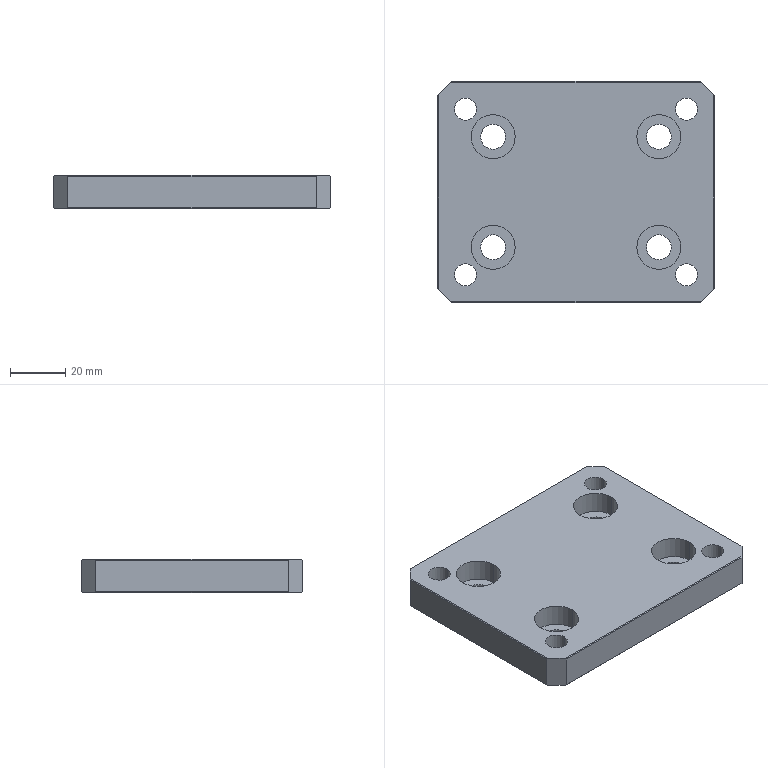Part | NX | 1 solid | 46 faces | box 100 x 80 x 12 mm | volume 85507 mm3 | cylinder 24 | plane 22 | commonest cylinder face diameters 8 x8 9 x8 16 x8
STEP:
#1=CARTESIAN_POINT('',(45.3,0.3,0.));
#2=VERTEX_POINT('',#1);
#3=CARTESIAN_POINT('',(-45.3,0.3,0.));
#4=VERTEX_POINT('',#3);
#5=CARTESIAN_POINT('',(0.,0.3,0.));
#6=DIRECTION('',(-1.,0.,0.));
#7=VECTOR('',#6,1000.);
#8=LINE('',#5,#7);
#9=EDGE_CURVE('',#2,#4,#8,.T.);
#10=ORIENTED_EDGE('',*,*,#9,.T.);
#11=CARTESIAN_POINT('',(-49.7,4.7,0.));
#12=VERTEX_POINT('',#11);
#13=CARTESIAN_POINT('',(-50.,5.,0.));
#14=DIRECTION('',(0.7071,-0.7071,0.));
#15=VECTOR('',#14,1000.);
#16=LINE('',#13,#15);
#17=EDGE_CURVE('',#12,#4,#16,.T.);
#18=ORIENTED_EDGE('',*,*,#17,.F.);
#19=CARTESIAN_POINT('',(-49.7,75.3,0.));
#20=VERTEX_POINT('',#19);
#21=CARTESIAN_POINT('',(-49.7,40.,0.));
#22=DIRECTION('',(0.,1.,0.));
#23=VECTOR('',#22,1000.);
#24=LINE('',#21,#23);
#25=EDGE_CURVE('',#12,#20,#24,.T.);
#26=ORIENTED_EDGE('',*,*,#25,.T.);
#27=CARTESIAN_POINT('',(-45.3,79.7,0.));
#28=VERTEX_POINT('',#27);
#29=CARTESIAN_POINT('',(-45.,80.,0.));
#30=DIRECTION('',(-0.7071,-0.7071,0.));
#31=VECTOR('',#30,1000.);
#32=LINE('',#29,#31);
#33=EDGE_CURVE('',#28,#20,#32,.T.);
#34=ORIENTED_EDGE('',*,*,#33,.F.);
#35=CARTESIAN_POINT('',(45.3,79.7,0.));
#36=VERTEX_POINT('',#35);
#37=CARTESIAN_POINT('',(0.,79.7,0.));
#38=DIRECTION('',(1.,0.,0.));
#39=VECTOR('',#38,1000.);
#40=LINE('',#37,#39);
#41=EDGE_CURVE('',#28,#36,#40,.T.);
#42=ORIENTED_EDGE('',*,*,#41,.T.);
#43=CARTESIAN_POINT('',(49.7,75.3,0.));
#44=VERTEX_POINT('',#43);
#45=CARTESIAN_POINT('',(50.,75.,0.));
#46=DIRECTION('',(-0.7071,0.7071,0.));
#47=VECTOR('',#46,1000.);
#48=LINE('',#45,#47);
#49=EDGE_CURVE('',#44,#36,#48,.T.);
#50=ORIENTED_EDGE('',*,*,#49,.F.);
#51=CARTESIAN_POINT('',(49.7,4.7,0.));
#52=VERTEX_POINT('',#51);
#53=CARTESIAN_POINT('',(49.7,40.,0.));
#54=DIRECTION('',(0.,-1.,0.));
#55=VECTOR('',#54,1000.);
#56=LINE('',#53,#55);
#57=EDGE_CURVE('',#44,#52,#56,.T.);
#58=ORIENTED_EDGE('',*,*,#57,.T.);
#59=CARTESIAN_POINT('',(45.,0.,0.));
#60=DIRECTION('',(0.7071,0.7071,0.));
#61=VECTOR('',#60,1000.);
#62=LINE('',#59,#61);
#63=EDGE_CURVE('',#2,#52,#62,.T.);
#64=ORIENTED_EDGE('',*,*,#63,.F.);
#65=EDGE_LOOP('',(#10,#18,#26,#34,#42,#50,#58,#64));
#66=FACE_BOUND('',#65,.T.);
#67=CARTESIAN_POINT('',(-34.5,60.,0.));
#68=VERTEX_POINT('',#67);
#69=CARTESIAN_POINT('',(-25.5,60.,0.));
#70=VERTEX_POINT('',#69);
#71=CARTESIAN_POINT('',(-30.,60.,0.));
#72=DIRECTION('',(0.,0.,-1.));
#73=DIRECTION('',(-1.,0.,0.));
#74=AXIS2_PLACEMENT_3D('',#71,#72,#73);
#75=CIRCLE('',#74,4.5);
#76=EDGE_CURVE('',#68,#70,#75,.T.);
#77=ORIENTED_EDGE('',*,*,#76,.F.);
#78=CARTESIAN_POINT('',(-30.,60.,0.));
#79=DIRECTION('',(0.,0.,-1.));
#80=DIRECTION('',(-1.,0.,0.));
#81=AXIS2_PLACEMENT_3D('',#78,#79,#80);
#82=CIRCLE('',#81,4.5);
#83=EDGE_CURVE('',#70,#68,#82,.T.);
#84=ORIENTED_EDGE('',*,*,#83,.F.);
#85=EDGE_LOOP('',(#77,#84));
#86=FACE_BOUND('',#85,.T.);
#87=CARTESIAN_POINT('',(25.5,20.,0.));
#88=VERTEX_POINT('',#87);
#89=CARTESIAN_POINT('',(34.5,20.,0.));
#90=VERTEX_POINT('',#89);
#91=CARTESIAN_POINT('',(30.,20.,0.));
#92=DIRECTION('',(0.,0.,-1.));
#93=DIRECTION('',(-1.,0.,0.));
#94=AXIS2_PLACEMENT_3D('',#91,#92,#93);
#95=CIRCLE('',#94,4.5);
#96=EDGE_CURVE('',#88,#90,#95,.T.);
#97=ORIENTED_EDGE('',*,*,#96,.F.);
#98=CARTESIAN_POINT('',(30.,20.,0.));
#99=DIRECTION('',(0.,0.,-1.));
#100=DIRECTION('',(-1.,0.,0.));
#101=AXIS2_PLACEMENT_3D('',#98,#99,#100);
#102=CIRCLE('',#101,4.5);
#103=EDGE_CURVE('',#90,#88,#102,.T.);
#104=ORIENTED_EDGE('',*,*,#103,.F.);
#105=EDGE_LOOP('',(#97,#104));
#106=FACE_BOUND('',#105,.T.);
#107=CARTESIAN_POINT('',(-25.5,20.,0.));
#108=VERTEX_POINT('',#107);
#109=CARTESIAN_POINT('',(-34.5,20.,0.));
#110=VERTEX_POINT('',#109);
#111=CARTESIAN_POINT('',(-30.,20.,0.));
#112=DIRECTION('',(0.,0.,-1.));
#113=DIRECTION('',(-1.,0.,0.));
#114=AXIS2_PLACEMENT_3D('',#111,#112,#113);
#115=CIRCLE('',#114,4.5);
#116=EDGE_CURVE('',#108,#110,#115,.T.);
#117=ORIENTED_EDGE('',*,*,#116,.F.);
#118=CARTESIAN_POINT('',(-30.,20.,0.));
#119=DIRECTION('',(0.,0.,-1.));
#120=DIRECTION('',(-1.,0.,0.));
#121=AXIS2_PLACEMENT_3D('',#118,#119,#120);
#122=CIRCLE('',#121,4.5);
#123=EDGE_CURVE('',#110,#108,#122,.T.);
#124=ORIENTED_EDGE('',*,*,#123,.F.);
#125=EDGE_LOOP('',(#117,#124));
#126=FACE_BOUND('',#125,.T.);
#127=CARTESIAN_POINT('',(36.,10.,0.));
#128=VERTEX_POINT('',#127);
#129=CARTESIAN_POINT('',(44.,10.,0.));
#130=VERTEX_POINT('',#129);
#131=CARTESIAN_POINT('',(40.,10.,0.));
#132=DIRECTION('',(0.,0.,-1.));
#133=DIRECTION('',(1.,0.,0.));
#134=AXIS2_PLACEMENT_3D('',#131,#132,#133);
#135=CIRCLE('',#134,4.);
#136=EDGE_CURVE('',#128,#130,#135,.T.);
#137=ORIENTED_EDGE('',*,*,#136,.F.);
#138=CARTESIAN_POINT('',(40.,10.,0.));
#139=DIRECTION('',(0.,0.,-1.));
#140=DIRECTION('',(1.,0.,0.));
#141=AXIS2_PLACEMENT_3D('',#138,#139,#140);
#142=CIRCLE('',#141,4.);
#143=EDGE_CURVE('',#130,#128,#142,.T.);
#144=ORIENTED_EDGE('',*,*,#143,.F.);
#145=EDGE_LOOP('',(#137,#144));
#146=FACE_BOUND('',#145,.T.);
#147=CARTESIAN_POINT('',(44.,70.,0.));
#148=VERTEX_POINT('',#147);
#149=CARTESIAN_POINT('',(36.,70.,0.));
#150=VERTEX_POINT('',#149);
#151=CARTESIAN_POINT('',(40.,70.,0.));
#152=DIRECTION('',(0.,0.,-1.));
#153=DIRECTION('',(1.,0.,0.));
#154=AXIS2_PLACEMENT_3D('',#151,#152,#153);
#155=CIRCLE('',#154,4.);
#156=EDGE_CURVE('',#148,#150,#155,.T.);
#157=ORIENTED_EDGE('',*,*,#156,.F.);
#158=CARTESIAN_POINT('',(40.,70.,0.));
#159=DIRECTION('',(0.,0.,-1.));
#160=DIRECTION('',(1.,0.,0.));
#161=AXIS2_PLACEMENT_3D('',#158,#159,#160);
#162=CIRCLE('',#161,4.);
#163=EDGE_CURVE('',#150,#148,#162,.T.);
#164=ORIENTED_EDGE('',*,*,#163,.F.);
#165=EDGE_LOOP('',(#157,#164));
#166=FACE_BOUND('',#165,.T.);
#167=CARTESIAN_POINT('',(-36.,10.,0.));
#168=VERTEX_POINT('',#167);
#169=CARTESIAN_POINT('',(-44.,10.,0.));
#170=VERTEX_POINT('',#169);
#171=CARTESIAN_POINT('',(-40.,10.,0.));
#172=DIRECTION('',(0.,0.,-1.));
#173=DIRECTION('',(1.,0.,0.));
#174=AXIS2_PLACEMENT_3D('',#171,#172,#173);
#175=CIRCLE('',#174,4.);
#176=EDGE_CURVE('',#168,#170,#175,.T.);
#177=ORIENTED_EDGE('',*,*,#176,.F.);
#178=CARTESIAN_POINT('',(-40.,10.,0.));
#179=DIRECTION('',(0.,0.,-1.));
#180=DIRECTION('',(1.,0.,0.));
#181=AXIS2_PLACEMENT_3D('',#178,#179,#180);
#182=CIRCLE('',#181,4.);
#183=EDGE_CURVE('',#170,#168,#182,.T.);
#184=ORIENTED_EDGE('',*,*,#183,.F.);
#185=EDGE_LOOP('',(#177,#184));
#186=FACE_BOUND('',#185,.T.);
#187=CARTESIAN_POINT('',(-44.,70.,0.));
#188=VERTEX_POINT('',#187);
#189=CARTESIAN_POINT('',(-36.,70.,0.));
#190=VERTEX_POINT('',#189);
#191=CARTESIAN_POINT('',(-40.,70.,0.));
#192=DIRECTION('',(0.,0.,-1.));
#193=DIRECTION('',(1.,0.,0.));
#194=AXIS2_PLACEMENT_3D('',#191,#192,#193);
#195=CIRCLE('',#194,4.);
#196=EDGE_CURVE('',#188,#190,#195,.T.);
#197=ORIENTED_EDGE('',*,*,#196,.F.);
#198=CARTESIAN_POINT('',(-40.,70.,0.));
#199=DIRECTION('',(0.,0.,-1.));
#200=DIRECTION('',(1.,0.,0.));
#201=AXIS2_PLACEMENT_3D('',#198,#199,#200);
#202=CIRCLE('',#201,4.);
#203=EDGE_CURVE('',#190,#188,#202,.T.);
#204=ORIENTED_EDGE('',*,*,#203,.F.);
#205=EDGE_LOOP('',(#197,#204));
#206=FACE_BOUND('',#205,.T.);
#207=CARTESIAN_POINT('',(34.5,60.,0.));
#208=VERTEX_POINT('',#207);
#209=CARTESIAN_POINT('',(25.5,60.,0.));
#210=VERTEX_POINT('',#209);
#211=CARTESIAN_POINT('',(30.,60.,0.));
#212=DIRECTION('',(0.,0.,-1.));
#213=DIRECTION('',(-1.,0.,0.));
#214=AXIS2_PLACEMENT_3D('',#211,#212,#213);
#215=CIRCLE('',#214,4.5);
#216=EDGE_CURVE('',#208,#210,#215,.T.);
#217=ORIENTED_EDGE('',*,*,#216,.F.);
#218=CARTESIAN_POINT('',(30.,60.,0.));
#219=DIRECTION('',(0.,0.,-1.));
#220=DIRECTION('',(-1.,0.,0.));
#221=AXIS2_PLACEMENT_3D('',#218,#219,#220);
#222=CIRCLE('',#221,4.5);
#223=EDGE_CURVE('',#210,#208,#222,.T.);
#224=ORIENTED_EDGE('',*,*,#223,.F.);
#225=EDGE_LOOP('',(#217,#224));
#226=FACE_BOUND('',#225,.T.);
#227=CARTESIAN_POINT('',(0.,0.,0.));
#228=DIRECTION('',(0.,0.,1.));
#229=DIRECTION('',(1.,0.,0.));
#230=AXIS2_PLACEMENT_3D('',#227,#228,#229);
#231=PLANE('',#230);
#232=ADVANCED_FACE('',(#66,#86,#106,#126,#146,#166,#186,#206,#226),#231,.F.);
#233=CARTESIAN_POINT('',(-50.,5.,0.3));
#234=VERTEX_POINT('',#233);
#235=CARTESIAN_POINT('',(-50.,75.,0.3));
#236=VERTEX_POINT('',#235);
#237=CARTESIAN_POINT('',(-50.,40.,0.3));
#238=DIRECTION('',(0.,1.,0.));
#239=VECTOR('',#238,1000.);
#240=LINE('',#237,#239);
#241=EDGE_CURVE('',#234,#236,#240,.T.);
#242=ORIENTED_EDGE('',*,*,#241,.F.);
#243=CARTESIAN_POINT('',(-50.,5.,11.7));
#244=VERTEX_POINT('',#243);
#245=CARTESIAN_POINT('',(-50.,5.,12.));
#246=DIRECTION('',(0.,0.,-1.));
#247=VECTOR('',#246,1000.);
#248=LINE('',#245,#247);
#249=EDGE_CURVE('',#244,#234,#248,.T.);
#250=ORIENTED_EDGE('',*,*,#249,.F.);
#251=CARTESIAN_POINT('',(-50.,75.,11.7));
#252=VERTEX_POINT('',#251);
#253=CARTESIAN_POINT('',(-50.,40.,11.7));
#254=DIRECTION('',(0.,1.,0.));
#255=VECTOR('',#254,1000.);
#256=LINE('',#253,#255);
#257=EDGE_CURVE('',#244,#252,#256,.T.);
#258=ORIENTED_EDGE('',*,*,#257,.T.);
#259=CARTESIAN_POINT('',(-50.,75.,12.));
#260=DIRECTION('',(0.,0.,-1.));
#261=VECTOR('',#260,1000.);
#262=LINE('',#259,#261);
#263=EDGE_CURVE('',#252,#236,#262,.T.);
#264=ORIENTED_EDGE('',*,*,#263,.T.);
#265=EDGE_LOOP('',(#242,#250,#258,#264));
#266=FACE_BOUND('',#265,.T.);
#267=CARTESIAN_POINT('',(-50.,80.,0.));
#268=DIRECTION('',(-1.,0.,0.));
#269=DIRECTION('',(0.,0.,1.));
#270=AXIS2_PLACEMENT_3D('',#267,#268,#269);
#271=PLANE('',#270);
#272=ADVANCED_FACE('',(#266),#271,.T.);
#273=ORIENTED_EDGE('',*,*,#263,.F.);
#274=CARTESIAN_POINT('',(-49.7,75.3,12.));
#275=VERTEX_POINT('',#274);
#276=CARTESIAN_POINT('',(-61.7,63.3,0.));
#277=DIRECTION('',(0.5774,0.5774,0.5774));
#278=VECTOR('',#277,1000.);
#279=LINE('',#276,#278);
#280=EDGE_CURVE('',#252,#275,#279,.T.);
#281=ORIENTED_EDGE('',*,*,#280,.T.);
#282=CARTESIAN_POINT('',(-45.3,79.7,12.));
#283=VERTEX_POINT('',#282);
#284=CARTESIAN_POINT('',(-50.,75.,12.));
#285=DIRECTION('',(0.7071,0.7071,0.));
#286=VECTOR('',#285,1000.);
#287=LINE('',#284,#286);
#288=EDGE_CURVE('',#275,#283,#287,.T.);
#289=ORIENTED_EDGE('',*,*,#288,.T.);
#290=CARTESIAN_POINT('',(-45.,80.,11.7));
#291=VERTEX_POINT('',#290);
#292=CARTESIAN_POINT('',(-33.3,91.7,0.));
#293=DIRECTION('',(0.5774,0.5774,-0.5774));
#294=VECTOR('',#293,1000.);
#295=LINE('',#292,#294);
#296=EDGE_CURVE('',#283,#291,#295,.T.);
#297=ORIENTED_EDGE('',*,*,#296,.T.);
#298=CARTESIAN_POINT('',(-45.,80.,0.3));
#299=VERTEX_POINT('',#298);
#300=CARTESIAN_POINT('',(-45.,80.,12.));
#301=DIRECTION('',(0.,0.,-1.));
#302=VECTOR('',#301,1000.);
#303=LINE('',#300,#302);
#304=EDGE_CURVE('',#291,#299,#303,.T.);
#305=ORIENTED_EDGE('',*,*,#304,.T.);
#306=CARTESIAN_POINT('',(-45.3,79.7,0.));
#307=DIRECTION('',(0.5774,0.5774,0.5774));
#308=VECTOR('',#307,1000.);
#309=LINE('',#306,#308);
#310=EDGE_CURVE('',#28,#299,#309,.T.);
#311=ORIENTED_EDGE('',*,*,#310,.F.);
#312=ORIENTED_EDGE('',*,*,#33,.T.);
#313=CARTESIAN_POINT('',(-49.7,75.3,0.));
#314=DIRECTION('',(0.5774,0.5774,-0.5774));
#315=VECTOR('',#314,1000.);
#316=LINE('',#313,#315);
#317=EDGE_CURVE('',#236,#20,#316,.T.);
#318=ORIENTED_EDGE('',*,*,#317,.F.);
#319=EDGE_LOOP('',(#273,#281,#289,#297,#305,#311,#312,#318));
#320=FACE_BOUND('',#319,.T.);
#321=CARTESIAN_POINT('',(-50.,75.,0.));
#322=DIRECTION('',(-0.7071,0.7071,0.));
#323=DIRECTION('',(0.,0.,1.));
#324=AXIS2_PLACEMENT_3D('',#321,#322,#323);
#325=PLANE('',#324);
#326=ADVANCED_FACE('',(#320),#325,.T.);
#327=CARTESIAN_POINT('',(45.,80.,0.3));
#328=VERTEX_POINT('',#327);
#329=CARTESIAN_POINT('',(0.,80.,0.3));
#330=DIRECTION('',(1.,0.,0.));
#331=VECTOR('',#330,1000.);
#332=LINE('',#329,#331);
#333=EDGE_CURVE('',#299,#328,#332,.T.);
#334=ORIENTED_EDGE('',*,*,#333,.F.);
#335=ORIENTED_EDGE('',*,*,#304,.F.);
#336=CARTESIAN_POINT('',(45.,80.,11.7));
#337=VERTEX_POINT('',#336);
#338=CARTESIAN_POINT('',(0.,80.,11.7));
#339=DIRECTION('',(1.,0.,0.));
#340=VECTOR('',#339,1000.);
#341=LINE('',#338,#340);
#342=EDGE_CURVE('',#291,#337,#341,.T.);
#343=ORIENTED_EDGE('',*,*,#342,.T.);
#344=CARTESIAN_POINT('',(45.,80.,12.));
#345=DIRECTION('',(0.,0.,-1.));
#346=VECTOR('',#345,1000.);
#347=LINE('',#344,#346);
#348=EDGE_CURVE('',#337,#328,#347,.T.);
#349=ORIENTED_EDGE('',*,*,#348,.T.);
#350=EDGE_LOOP('',(#334,#335,#343,#349));
#351=FACE_BOUND('',#350,.T.);
#352=CARTESIAN_POINT('',(50.,80.,0.));
#353=DIRECTION('',(0.,1.,0.));
#354=DIRECTION('',(1.,0.,0.));
#355=AXIS2_PLACEMENT_3D('',#352,#353,#354);
#356=PLANE('',#355);
#357=ADVANCED_FACE('',(#351),#356,.T.);
#358=ORIENTED_EDGE('',*,*,#348,.F.);
#359=CARTESIAN_POINT('',(45.3,79.7,12.));
#360=VERTEX_POINT('',#359);
#361=CARTESIAN_POINT('',(33.3,91.7,0.));
#362=DIRECTION('',(0.5774,-0.5774,0.5774));
#363=VECTOR('',#362,1000.);
#364=LINE('',#361,#363);
#365=EDGE_CURVE('',#337,#360,#364,.T.);
#366=ORIENTED_EDGE('',*,*,#365,.T.);
#367=CARTESIAN_POINT('',(49.7,75.3,12.));
#368=VERTEX_POINT('',#367);
#369=CARTESIAN_POINT('',(45.,80.,12.));
#370=DIRECTION('',(0.7071,-0.7071,0.));
#371=VECTOR('',#370,1000.);
#372=LINE('',#369,#371);
#373=EDGE_CURVE('',#360,#368,#372,.T.);
#374=ORIENTED_EDGE('',*,*,#373,.T.);
#375=CARTESIAN_POINT('',(50.,75.,11.7));
#376=VERTEX_POINT('',#375);
#377=CARTESIAN_POINT('',(61.7,63.3,0.));
#378=DIRECTION('',(0.5774,-0.5774,-0.5774));
#379=VECTOR('',#378,1000.);
#380=LINE('',#377,#379);
#381=EDGE_CURVE('',#368,#376,#380,.T.);
#382=ORIENTED_EDGE('',*,*,#381,.T.);
#383=CARTESIAN_POINT('',(50.,75.,0.3));
#384=VERTEX_POINT('',#383);
#385=CARTESIAN_POINT('',(50.,75.,12.));
#386=DIRECTION('',(0.,0.,-1.));
#387=VECTOR('',#386,1000.);
#388=LINE('',#385,#387);
#389=EDGE_CURVE('',#376,#384,#388,.T.);
#390=ORIENTED_EDGE('',*,*,#389,.T.);
#391=CARTESIAN_POINT('',(49.7,75.3,0.));
#392=DIRECTION('',(0.5774,-0.5774,0.5774));
#393=VECTOR('',#392,1000.);
#394=LINE('',#391,#393);
#395=EDGE_CURVE('',#44,#384,#394,.T.);
#396=ORIENTED_EDGE('',*,*,#395,.F.);
#397=ORIENTED_EDGE('',*,*,#49,.T.);
#398=CARTESIAN_POINT('',(45.3,79.7,0.));
#399=DIRECTION('',(0.5774,-0.5774,-0.5774));
#400=VECTOR('',#399,1000.);
#401=LINE('',#398,#400);
#402=EDGE_CURVE('',#328,#36,#401,.T.);
#403=ORIENTED_EDGE('',*,*,#402,.F.);
#404=EDGE_LOOP('',(#358,#366,#374,#382,#390,#396,#397,#403));
#405=FACE_BOUND('',#404,.T.);
#406=CARTESIAN_POINT('',(45.,80.,0.));
#407=DIRECTION('',(0.7071,0.7071,0.));
#408=DIRECTION('',(0.,0.,-1.));
#409=AXIS2_PLACEMENT_3D('',#406,#407,#408);
#410=PLANE('',#409);
#411=ADVANCED_FACE('',(#405),#410,.T.);
#412=CARTESIAN_POINT('',(50.,5.,0.3));
#413=VERTEX_POINT('',#412);
#414=CARTESIAN_POINT('',(50.,40.,0.3));
#415=DIRECTION('',(0.,-1.,0.));
#416=VECTOR('',#415,1000.);
#417=LINE('',#414,#416);
#418=EDGE_CURVE('',#384,#413,#417,.T.);
#419=ORIENTED_EDGE('',*,*,#418,.F.);
#420=ORIENTED_EDGE('',*,*,#389,.F.);
#421=CARTESIAN_POINT('',(50.,5.,11.7));
#422=VERTEX_POINT('',#421);
#423=CARTESIAN_POINT('',(50.,40.,11.7));
#424=DIRECTION('',(0.,-1.,0.));
#425=VECTOR('',#424,1000.);
#426=LINE('',#423,#425);
#427=EDGE_CURVE('',#376,#422,#426,.T.);
#428=ORIENTED_EDGE('',*,*,#427,.T.);
#429=CARTESIAN_POINT('',(50.,5.,12.));
#430=DIRECTION('',(0.,0.,-1.));
#431=VECTOR('',#430,1000.);
#432=LINE('',#429,#431);
#433=EDGE_CURVE('',#422,#413,#432,.T.);
#434=ORIENTED_EDGE('',*,*,#433,.T.);
#435=EDGE_LOOP('',(#419,#420,#428,#434));
#436=FACE_BOUND('',#435,.T.);
#437=CARTESIAN_POINT('',(50.,0.,0.));
#438=DIRECTION('',(1.,0.,0.));
#439=DIRECTION('',(0.,1.,0.));
#440=AXIS2_PLACEMENT_3D('',#437,#438,#439);
#441=PLANE('',#440);
#442=ADVANCED_FACE('',(#436),#441,.T.);
#443=ORIENTED_EDGE('',*,*,#433,.F.);
#444=CARTESIAN_POINT('',(49.7,4.7,12.));
#445=VERTEX_POINT('',#444);
#446=CARTESIAN_POINT('',(61.7,16.7,0.));
#447=DIRECTION('',(-0.5774,-0.5774,0.5774));
#448=VECTOR('',#447,1000.);
#449=LINE('',#446,#448);
#450=EDGE_CURVE('',#422,#445,#449,.T.);
#451=ORIENTED_EDGE('',*,*,#450,.T.);
#452=CARTESIAN_POINT('',(45.3,0.3,12.));
#453=VERTEX_POINT('',#452);
#454=CARTESIAN_POINT('',(50.,5.,12.));
#455=DIRECTION('',(-0.7071,-0.7071,0.));
#456=VECTOR('',#455,1000.);
#457=LINE('',#454,#456);
#458=EDGE_CURVE('',#445,#453,#457,.T.);
#459=ORIENTED_EDGE('',*,*,#458,.T.);
#460=CARTESIAN_POINT('',(45.,0.,11.7));
#461=VERTEX_POINT('',#460);
#462=CARTESIAN_POINT('',(33.3,-11.7,0.));
#463=DIRECTION('',(-0.5774,-0.5774,-0.5774));
#464=VECTOR('',#463,1000.);
#465=LINE('',#462,#464);
#466=EDGE_CURVE('',#453,#461,#465,.T.);
#467=ORIENTED_EDGE('',*,*,#466,.T.);
#468=CARTESIAN_POINT('',(45.,0.,0.3));
#469=VERTEX_POINT('',#468);
#470=CARTESIAN_POINT('',(45.,0.,12.));
#471=DIRECTION('',(0.,0.,-1.));
#472=VECTOR('',#471,1000.);
#473=LINE('',#470,#472);
#474=EDGE_CURVE('',#461,#469,#473,.T.);
#475=ORIENTED_EDGE('',*,*,#474,.T.);
#476=CARTESIAN_POINT('',(45.3,0.3,0.));
#477=DIRECTION('',(-0.5774,-0.5774,0.5774));
#478=VECTOR('',#477,1000.);
#479=LINE('',#476,#478);
#480=EDGE_CURVE('',#2,#469,#479,.T.);
#481=ORIENTED_EDGE('',*,*,#480,.F.);
#482=ORIENTED_EDGE('',*,*,#63,.T.);
#483=CARTESIAN_POINT('',(49.7,4.7,0.));
#484=DIRECTION('',(-0.5774,-0.5774,-0.5774));
#485=VECTOR('',#484,1000.);
#486=LINE('',#483,#485);
#487=EDGE_CURVE('',#413,#52,#486,.T.);
#488=ORIENTED_EDGE('',*,*,#487,.F.);
#489=EDGE_LOOP('',(#443,#451,#459,#467,#475,#481,#482,#488));
#490=FACE_BOUND('',#489,.T.);
#491=CARTESIAN_POINT('',(50.,5.,0.));
#492=DIRECTION('',(0.7071,-0.7071,0.));
#493=DIRECTION('',(0.,0.,-1.));
#494=AXIS2_PLACEMENT_3D('',#491,#492,#493);
#495=PLANE('',#494);
#496=ADVANCED_FACE('',(#490),#495,.T.);
#497=CARTESIAN_POINT('',(-45.,0.,0.3));
#498=VERTEX_POINT('',#497);
#499=CARTESIAN_POINT('',(0.,0.,0.3));
#500=DIRECTION('',(-1.,0.,0.));
#501=VECTOR('',#500,1000.);
#502=LINE('',#499,#501);
#503=EDGE_CURVE('',#469,#498,#502,.T.);
#504=ORIENTED_EDGE('',*,*,#503,.F.);
#505=ORIENTED_EDGE('',*,*,#474,.F.);
#506=CARTESIAN_POINT('',(-45.,0.,11.7));
#507=VERTEX_POINT('',#506);
#508=CARTESIAN_POINT('',(0.,0.,11.7));
#509=DIRECTION('',(-1.,0.,0.));
#510=VECTOR('',#509,1000.);
#511=LINE('',#508,#510);
#512=EDGE_CURVE('',#461,#507,#511,.T.);
#513=ORIENTED_EDGE('',*,*,#512,.T.);
#514=CARTESIAN_POINT('',(-45.,0.,12.));
#515=DIRECTION('',(0.,0.,-1.));
#516=VECTOR('',#515,1000.);
#517=LINE('',#514,#516);
#518=EDGE_CURVE('',#507,#498,#517,.T.);
#519=ORIENTED_EDGE('',*,*,#518,.T.);
#520=EDGE_LOOP('',(#504,#505,#513,#519));
#521=FACE_BOUND('',#520,.T.);
#522=CARTESIAN_POINT('',(-50.,0.,0.));
#523=DIRECTION('',(0.,-1.,0.));
#524=DIRECTION('',(0.,0.,-1.));
#525=AXIS2_PLACEMENT_3D('',#522,#523,#524);
#526=PLANE('',#525);
#527=ADVANCED_FACE('',(#521),#526,.T.);
#528=ORIENTED_EDGE('',*,*,#518,.F.);
#529=CARTESIAN_POINT('',(-45.3,0.3,12.));
#530=VERTEX_POINT('',#529);
#531=CARTESIAN_POINT('',(-33.3,-11.7,0.));
#532=DIRECTION('',(-0.5774,0.5774,0.5774));
#533=VECTOR('',#532,1000.);
#534=LINE('',#531,#533);
#535=EDGE_CURVE('',#507,#530,#534,.T.);
#536=ORIENTED_EDGE('',*,*,#535,.T.);
#537=CARTESIAN_POINT('',(-49.7,4.7,12.));
#538=VERTEX_POINT('',#537);
#539=CARTESIAN_POINT('',(-45.,0.,12.));
#540=DIRECTION('',(-0.7071,0.7071,0.));
#541=VECTOR('',#540,1000.);
#542=LINE('',#539,#541);
#543=EDGE_CURVE('',#530,#538,#542,.T.);
#544=ORIENTED_EDGE('',*,*,#543,.T.);
#545=CARTESIAN_POINT('',(-61.7,16.7,0.));
#546=DIRECTION('',(-0.5774,0.5774,-0.5774));
#547=VECTOR('',#546,1000.);
#548=LINE('',#545,#547);
#549=EDGE_CURVE('',#538,#244,#548,.T.);
#550=ORIENTED_EDGE('',*,*,#549,.T.);
#551=ORIENTED_EDGE('',*,*,#249,.T.);
#552=CARTESIAN_POINT('',(-49.7,4.7,0.));
#553=DIRECTION('',(-0.5774,0.5774,0.5774));
#554=VECTOR('',#553,1000.);
#555=LINE('',#552,#554);
#556=EDGE_CURVE('',#12,#234,#555,.T.);
#557=ORIENTED_EDGE('',*,*,#556,.F.);
#558=ORIENTED_EDGE('',*,*,#17,.T.);
#559=CARTESIAN_POINT('',(-45.3,0.3,0.));
#560=DIRECTION('',(-0.5774,0.5774,-0.5774));
#561=VECTOR('',#560,1000.);
#562=LINE('',#559,#561);
#563=EDGE_CURVE('',#498,#4,#562,.T.);
#564=ORIENTED_EDGE('',*,*,#563,.F.);
#565=EDGE_LOOP('',(#528,#536,#544,#550,#551,#557,#558,#564));
#566=FACE_BOUND('',#565,.T.);
#567=CARTESIAN_POINT('',(-45.,0.,0.));
#568=DIRECTION('',(-0.7071,-0.7071,0.));
#569=DIRECTION('',(-0.7071,0.7071,0.));
#570=AXIS2_PLACEMENT_3D('',#567,#568,#569);
#571=PLANE('',#570);
#572=ADVANCED_FACE('',(#566),#571,.T.);
#573=CARTESIAN_POINT('',(0.,0.3,12.));
#574=DIRECTION('',(-1.,0.,0.));
#575=VECTOR('',#574,1000.);
#576=LINE('',#573,#575);
#577=EDGE_CURVE('',#453,#530,#576,.T.);
#578=ORIENTED_EDGE('',*,*,#577,.F.);
#579=ORIENTED_EDGE('',*,*,#458,.F.);
#580=CARTESIAN_POINT('',(49.7,40.,12.));
#581=DIRECTION('',(0.,-1.,0.));
#582=VECTOR('',#581,1000.);
#583=LINE('',#580,#582);
#584=EDGE_CURVE('',#368,#445,#583,.T.);
#585=ORIENTED_EDGE('',*,*,#584,.F.);
#586=ORIENTED_EDGE('',*,*,#373,.F.);
#587=CARTESIAN_POINT('',(0.,79.7,12.));
#588=DIRECTION('',(1.,0.,0.));
#589=VECTOR('',#588,1000.);
#590=LINE('',#587,#589);
#591=EDGE_CURVE('',#283,#360,#590,.T.);
#592=ORIENTED_EDGE('',*,*,#591,.F.);
#593=ORIENTED_EDGE('',*,*,#288,.F.);
#594=CARTESIAN_POINT('',(-49.7,40.,12.));
#595=DIRECTION('',(0.,1.,0.));
#596=VECTOR('',#595,1000.);
#597=LINE('',#594,#596);
#598=EDGE_CURVE('',#538,#275,#597,.T.);
#599=ORIENTED_EDGE('',*,*,#598,.F.);
#600=ORIENTED_EDGE('',*,*,#543,.F.);
#601=EDGE_LOOP('',(#578,#579,#585,#586,#592,#593,#599,#600));
#602=FACE_BOUND('',#601,.T.);
#603=CARTESIAN_POINT('',(-38.,60.,12.));
#604=VERTEX_POINT('',#603);
#605=CARTESIAN_POINT('',(-22.,60.,12.));
#606=VERTEX_POINT('',#605);
#607=CARTESIAN_POINT('',(-30.,60.,12.));
#608=DIRECTION('',(0.,0.,1.));
#609=DIRECTION('',(1.,0.,0.));
#610=AXIS2_PLACEMENT_3D('',#607,#608,#609);
#611=CIRCLE('',#610,8.);
#612=EDGE_CURVE('',#604,#606,#611,.T.);
#613=ORIENTED_EDGE('',*,*,#612,.F.);
#614=CARTESIAN_POINT('',(-30.,60.,12.));
#615=DIRECTION('',(0.,0.,1.));
#616=DIRECTION('',(1.,0.,0.));
#617=AXIS2_PLACEMENT_3D('',#614,#615,#616);
#618=CIRCLE('',#617,8.);
#619=EDGE_CURVE('',#606,#604,#618,.T.);
#620=ORIENTED_EDGE('',*,*,#619,.F.);
#621=EDGE_LOOP('',(#613,#620));
#622=FACE_BOUND('',#621,.T.);
#623=CARTESIAN_POINT('',(38.,20.,12.));
#624=VERTEX_POINT('',#623);
#625=CARTESIAN_POINT('',(22.,20.,12.));
#626=VERTEX_POINT('',#625);
#627=CARTESIAN_POINT('',(30.,20.,12.));
#628=DIRECTION('',(0.,0.,1.));
#629=DIRECTION('',(1.,0.,0.));
#630=AXIS2_PLACEMENT_3D('',#627,#628,#629);
#631=CIRCLE('',#630,8.);
#632=EDGE_CURVE('',#624,#626,#631,.T.);
#633=ORIENTED_EDGE('',*,*,#632,.F.);
#634=CARTESIAN_POINT('',(30.,20.,12.));
#635=DIRECTION('',(0.,0.,1.));
#636=DIRECTION('',(1.,0.,0.));
#637=AXIS2_PLACEMENT_3D('',#634,#635,#636);
#638=CIRCLE('',#637,8.);
#639=EDGE_CURVE('',#626,#624,#638,.T.);
#640=ORIENTED_EDGE('',*,*,#639,.F.);
#641=EDGE_LOOP('',(#633,#640));
#642=FACE_BOUND('',#641,.T.);
#643=CARTESIAN_POINT('',(-38.,20.,12.));
#644=VERTEX_POINT('',#643);
#645=CARTESIAN_POINT('',(-22.,20.,12.));
#646=VERTEX_POINT('',#645);
#647=CARTESIAN_POINT('',(-30.,20.,12.));
#648=DIRECTION('',(0.,0.,1.));
#649=DIRECTION('',(1.,0.,0.));
#650=AXIS2_PLACEMENT_3D('',#647,#648,#649);
#651=CIRCLE('',#650,8.);
#652=EDGE_CURVE('',#644,#646,#651,.T.);
#653=ORIENTED_EDGE('',*,*,#652,.F.);
#654=CARTESIAN_POINT('',(-30.,20.,12.));
#655=DIRECTION('',(0.,0.,1.));
#656=DIRECTION('',(1.,0.,0.));
#657=AXIS2_PLACEMENT_3D('',#654,#655,#656);
#658=CIRCLE('',#657,8.);
#659=EDGE_CURVE('',#646,#644,#658,.T.);
#660=ORIENTED_EDGE('',*,*,#659,.F.);
#661=EDGE_LOOP('',(#653,#660));
#662=FACE_BOUND('',#661,.T.);
#663=CARTESIAN_POINT('',(44.,10.,12.));
#664=VERTEX_POINT('',#663);
#665=CARTESIAN_POINT('',(36.,10.,12.));
#666=VERTEX_POINT('',#665);
#667=CARTESIAN_POINT('',(40.,10.,12.));
#668=DIRECTION('',(0.,0.,1.));
#669=DIRECTION('',(-1.,0.,0.));
#670=AXIS2_PLACEMENT_3D('',#667,#668,#669);
#671=CIRCLE('',#670,4.);
#672=EDGE_CURVE('',#664,#666,#671,.T.);
#673=ORIENTED_EDGE('',*,*,#672,.F.);
#674=CARTESIAN_POINT('',(40.,10.,12.));
#675=DIRECTION('',(0.,0.,1.));
#676=DIRECTION('',(-1.,0.,0.));
#677=AXIS2_PLACEMENT_3D('',#674,#675,#676);
#678=CIRCLE('',#677,4.);
#679=EDGE_CURVE('',#666,#664,#678,.T.);
#680=ORIENTED_EDGE('',*,*,#679,.F.);
#681=EDGE_LOOP('',(#673,#680));
#682=FACE_BOUND('',#681,.T.);
#683=CARTESIAN_POINT('',(44.,70.,12.));
#684=VERTEX_POINT('',#683);
#685=CARTESIAN_POINT('',(36.,70.,12.));
#686=VERTEX_POINT('',#685);
#687=CARTESIAN_POINT('',(40.,70.,12.));
#688=DIRECTION('',(0.,0.,1.));
#689=DIRECTION('',(-1.,0.,0.));
#690=AXIS2_PLACEMENT_3D('',#687,#688,#689);
#691=CIRCLE('',#690,4.);
#692=EDGE_CURVE('',#684,#686,#691,.T.);
#693=ORIENTED_EDGE('',*,*,#692,.F.);
#694=CARTESIAN_POINT('',(40.,70.,12.));
#695=DIRECTION('',(0.,0.,1.));
#696=DIRECTION('',(-1.,0.,0.));
#697=AXIS2_PLACEMENT_3D('',#694,#695,#696);
#698=CIRCLE('',#697,4.);
#699=EDGE_CURVE('',#686,#684,#698,.T.);
#700=ORIENTED_EDGE('',*,*,#699,.F.);
#701=EDGE_LOOP('',(#693,#700));
#702=FACE_BOUND('',#701,.T.);
#703=CARTESIAN_POINT('',(-44.,10.,12.));
#704=VERTEX_POINT('',#703);
#705=CARTESIAN_POINT('',(-36.,10.,12.));
#706=VERTEX_POINT('',#705);
#707=CARTESIAN_POINT('',(-40.,10.,12.));
#708=DIRECTION('',(0.,0.,1.));
#709=DIRECTION('',(-1.,0.,0.));
#710=AXIS2_PLACEMENT_3D('',#707,#708,#709);
#711=CIRCLE('',#710,4.);
#712=EDGE_CURVE('',#704,#706,#711,.T.);
#713=ORIENTED_EDGE('',*,*,#712,.F.);
#714=CARTESIAN_POINT('',(-40.,10.,12.));
#715=DIRECTION('',(0.,0.,1.));
#716=DIRECTION('',(-1.,0.,0.));
#717=AXIS2_PLACEMENT_3D('',#714,#715,#716);
#718=CIRCLE('',#717,4.);
#719=EDGE_CURVE('',#706,#704,#718,.T.);
#720=ORIENTED_EDGE('',*,*,#719,.F.);
#721=EDGE_LOOP('',(#713,#720));
#722=FACE_BOUND('',#721,.T.);
#723=CARTESIAN_POINT('',(-44.,70.,12.));
#724=VERTEX_POINT('',#723);
#725=CARTESIAN_POINT('',(-36.,70.,12.));
#726=VERTEX_POINT('',#725);
#727=CARTESIAN_POINT('',(-40.,70.,12.));
#728=DIRECTION('',(0.,0.,1.));
#729=DIRECTION('',(-1.,0.,0.));
#730=AXIS2_PLACEMENT_3D('',#727,#728,#729);
#731=CIRCLE('',#730,4.);
#732=EDGE_CURVE('',#724,#726,#731,.T.);
#733=ORIENTED_EDGE('',*,*,#732,.F.);
#734=CARTESIAN_POINT('',(-40.,70.,12.));
#735=DIRECTION('',(0.,0.,1.));
#736=DIRECTION('',(-1.,0.,0.));
#737=AXIS2_PLACEMENT_3D('',#734,#735,#736);
#738=CIRCLE('',#737,4.);
#739=EDGE_CURVE('',#726,#724,#738,.T.);
#740=ORIENTED_EDGE('',*,*,#739,.F.);
#741=EDGE_LOOP('',(#733,#740));
#742=FACE_BOUND('',#741,.T.);
#743=CARTESIAN_POINT('',(38.,60.,12.));
#744=VERTEX_POINT('',#743);
#745=CARTESIAN_POINT('',(22.,60.,12.));
#746=VERTEX_POINT('',#745);
#747=CARTESIAN_POINT('',(30.,60.,12.));
#748=DIRECTION('',(0.,0.,1.));
#749=DIRECTION('',(1.,0.,0.));
#750=AXIS2_PLACEMENT_3D('',#747,#748,#749);
#751=CIRCLE('',#750,8.);
#752=EDGE_CURVE('',#744,#746,#751,.T.);
#753=ORIENTED_EDGE('',*,*,#752,.F.);
#754=CARTESIAN_POINT('',(30.,60.,12.));
#755=DIRECTION('',(0.,0.,1.));
#756=DIRECTION('',(1.,0.,0.));
#757=AXIS2_PLACEMENT_3D('',#754,#755,#756);
#758=CIRCLE('',#757,8.);
#759=EDGE_CURVE('',#746,#744,#758,.T.);
#760=ORIENTED_EDGE('',*,*,#759,.F.);
#761=EDGE_LOOP('',(#753,#760));
#762=FACE_BOUND('',#761,.T.);
#763=CARTESIAN_POINT('',(0.,0.,12.));
#764=DIRECTION('',(0.,0.,1.));
#765=DIRECTION('',(1.,0.,0.));
#766=AXIS2_PLACEMENT_3D('',#763,#764,#765);
#767=PLANE('',#766);
#768=ADVANCED_FACE('',(#602,#622,#642,#662,#682,#702,#722,#742,#762),#767,.T.);
#769=CARTESIAN_POINT('',(22.,60.,4.));
#770=VERTEX_POINT('',#769);
#771=CARTESIAN_POINT('',(38.,60.,4.));
#772=VERTEX_POINT('',#771);
#773=CARTESIAN_POINT('',(30.,60.,4.));
#774=DIRECTION('',(0.,0.,-1.));
#775=DIRECTION('',(1.,0.,0.));
#776=AXIS2_PLACEMENT_3D('',#773,#774,#775);
#777=CIRCLE('',#776,8.);
#778=EDGE_CURVE('',#770,#772,#777,.T.);
#779=ORIENTED_EDGE('',*,*,#778,.T.);
#780=CARTESIAN_POINT('',(38.,60.,-1.86));
#781=DIRECTION('',(0.,0.,1.));
#782=VECTOR('',#781,1000.);
#783=LINE('',#780,#782);
#784=EDGE_CURVE('',#744,#772,#783,.F.);
#785=ORIENTED_EDGE('',*,*,#784,.F.);
#786=ORIENTED_EDGE('',*,*,#752,.T.);
#787=CARTESIAN_POINT('',(22.,60.,-1.86));
#788=DIRECTION('',(0.,0.,1.));
#789=VECTOR('',#788,1000.);
#790=LINE('',#787,#789);
#791=EDGE_CURVE('',#746,#770,#790,.F.);
#792=ORIENTED_EDGE('',*,*,#791,.T.);
#793=EDGE_LOOP('',(#779,#785,#786,#792));
#794=FACE_BOUND('',#793,.T.);
#795=CARTESIAN_POINT('',(30.,60.,-1.86));
#796=DIRECTION('',(0.,0.,1.));
#797=DIRECTION('',(-1.,0.,0.));
#798=AXIS2_PLACEMENT_3D('',#795,#796,#797);
#799=CYLINDRICAL_SURFACE('',#798,8.);
#800=ADVANCED_FACE('',(#794),#799,.F.);
#801=ORIENTED_EDGE('',*,*,#136,.T.);
#802=CARTESIAN_POINT('',(44.,10.,12.));
#803=DIRECTION('',(0.,0.,-1.));
#804=VECTOR('',#803,1000.);
#805=LINE('',#802,#804);
#806=EDGE_CURVE('',#130,#664,#805,.F.);
#807=ORIENTED_EDGE('',*,*,#806,.T.);
#808=ORIENTED_EDGE('',*,*,#672,.T.);
#809=CARTESIAN_POINT('',(36.,10.,12.));
#810=DIRECTION('',(0.,0.,-1.));
#811=VECTOR('',#810,1000.);
#812=LINE('',#809,#811);
#813=EDGE_CURVE('',#128,#666,#812,.F.);
#814=ORIENTED_EDGE('',*,*,#813,.F.);
#815=EDGE_LOOP('',(#801,#807,#808,#814));
#816=FACE_BOUND('',#815,.T.);
#817=CARTESIAN_POINT('',(40.,10.,12.));
#818=DIRECTION('',(0.,0.,-1.));
#819=DIRECTION('',(-1.,0.,0.));
#820=AXIS2_PLACEMENT_3D('',#817,#818,#819);
#821=CYLINDRICAL_SURFACE('',#820,4.);
#822=ADVANCED_FACE('',(#816),#821,.F.);
#823=ORIENTED_EDGE('',*,*,#778,.F.);
#824=CARTESIAN_POINT('',(30.,60.,4.));
#825=DIRECTION('',(0.,0.,-1.));
#826=DIRECTION('',(1.,0.,0.));
#827=AXIS2_PLACEMENT_3D('',#824,#825,#826);
#828=CIRCLE('',#827,8.);
#829=EDGE_CURVE('',#772,#770,#828,.T.);
#830=ORIENTED_EDGE('',*,*,#829,.F.);
#831=EDGE_LOOP('',(#823,#830));
#832=FACE_BOUND('',#831,.T.);
#833=CARTESIAN_POINT('',(25.5,60.,4.));
#834=VERTEX_POINT('',#833);
#835=CARTESIAN_POINT('',(34.5,60.,4.));
#836=VERTEX_POINT('',#835);
#837=CARTESIAN_POINT('',(30.,60.,4.));
#838=DIRECTION('',(0.,0.,1.));
#839=DIRECTION('',(-1.,0.,0.));
#840=AXIS2_PLACEMENT_3D('',#837,#838,#839);
#841=CIRCLE('',#840,4.5);
#842=EDGE_CURVE('',#834,#836,#841,.T.);
#843=ORIENTED_EDGE('',*,*,#842,.F.);
#844=CARTESIAN_POINT('',(30.,60.,4.));
#845=DIRECTION('',(0.,0.,1.));
#846=DIRECTION('',(-1.,0.,0.));
#847=AXIS2_PLACEMENT_3D('',#844,#845,#846);
#848=CIRCLE('',#847,4.5);
#849=EDGE_CURVE('',#836,#834,#848,.T.);
#850=ORIENTED_EDGE('',*,*,#849,.F.);
#851=EDGE_LOOP('',(#843,#850));
#852=FACE_BOUND('',#851,.T.);
#853=CARTESIAN_POINT('',(30.,60.,4.));
#854=DIRECTION('',(0.,0.,1.));
#855=DIRECTION('',(1.,0.,0.));
#856=AXIS2_PLACEMENT_3D('',#853,#854,#855);
#857=PLANE('',#856);
#858=ADVANCED_FACE('',(#832,#852),#857,.T.);
#859=ORIENTED_EDGE('',*,*,#842,.T.);
#860=CARTESIAN_POINT('',(34.5,60.,-1.86));
#861=DIRECTION('',(0.,0.,1.));
#862=VECTOR('',#861,1000.);
#863=LINE('',#860,#862);
#864=EDGE_CURVE('',#836,#208,#863,.F.);
#865=ORIENTED_EDGE('',*,*,#864,.T.);
#866=ORIENTED_EDGE('',*,*,#216,.T.);
#867=CARTESIAN_POINT('',(25.5,60.,-1.86));
#868=DIRECTION('',(0.,0.,1.));
#869=VECTOR('',#868,1000.);
#870=LINE('',#867,#869);
#871=EDGE_CURVE('',#834,#210,#870,.F.);
#872=ORIENTED_EDGE('',*,*,#871,.F.);
#873=EDGE_LOOP('',(#859,#865,#866,#872));
#874=FACE_BOUND('',#873,.T.);
#875=CARTESIAN_POINT('',(30.,60.,-1.86));
#876=DIRECTION('',(0.,0.,1.));
#877=DIRECTION('',(-1.,0.,0.));
#878=AXIS2_PLACEMENT_3D('',#875,#876,#877);
#879=CYLINDRICAL_SURFACE('',#878,4.5);
#880=ADVANCED_FACE('',(#874),#879,.F.);
#881=ORIENTED_EDGE('',*,*,#712,.T.);
#882=CARTESIAN_POINT('',(-36.,10.,12.));
#883=DIRECTION('',(0.,0.,-1.));
#884=VECTOR('',#883,1000.);
#885=LINE('',#882,#884);
#886=EDGE_CURVE('',#168,#706,#885,.F.);
#887=ORIENTED_EDGE('',*,*,#886,.F.);
#888=ORIENTED_EDGE('',*,*,#176,.T.);
#889=CARTESIAN_POINT('',(-44.,10.,12.));
#890=DIRECTION('',(0.,0.,-1.));
#891=VECTOR('',#890,1000.);
#892=LINE('',#889,#891);
#893=EDGE_CURVE('',#170,#704,#892,.F.);
#894=ORIENTED_EDGE('',*,*,#893,.T.);
#895=EDGE_LOOP('',(#881,#887,#888,#894));
#896=FACE_BOUND('',#895,.T.);
#897=CARTESIAN_POINT('',(-40.,10.,12.));
#898=DIRECTION('',(0.,0.,-1.));
#899=DIRECTION('',(-1.,0.,0.));
#900=AXIS2_PLACEMENT_3D('',#897,#898,#899);
#901=CYLINDRICAL_SURFACE('',#900,4.);
#902=ADVANCED_FACE('',(#896),#901,.F.);
#903=ORIENTED_EDGE('',*,*,#612,.T.);
#904=CARTESIAN_POINT('',(-22.,60.,4.));
#905=VERTEX_POINT('',#904);
#906=CARTESIAN_POINT('',(-22.,60.,-1.86));
#907=DIRECTION('',(0.,0.,1.));
#908=VECTOR('',#907,1000.);
#909=LINE('',#906,#908);
#910=EDGE_CURVE('',#905,#606,#909,.T.);
#911=ORIENTED_EDGE('',*,*,#910,.F.);
#912=CARTESIAN_POINT('',(-38.,60.,4.));
#913=VERTEX_POINT('',#912);
#914=CARTESIAN_POINT('',(-30.,60.,4.));
#915=DIRECTION('',(0.,0.,-1.));
#916=DIRECTION('',(1.,0.,0.));
#917=AXIS2_PLACEMENT_3D('',#914,#915,#916);
#918=CIRCLE('',#917,8.);
#919=EDGE_CURVE('',#905,#913,#918,.T.);
#920=ORIENTED_EDGE('',*,*,#919,.T.);
#921=CARTESIAN_POINT('',(-38.,60.,-1.86));
#922=DIRECTION('',(0.,0.,1.));
#923=VECTOR('',#922,1000.);
#924=LINE('',#921,#923);
#925=EDGE_CURVE('',#913,#604,#924,.T.);
#926=ORIENTED_EDGE('',*,*,#925,.T.);
#927=EDGE_LOOP('',(#903,#911,#920,#926));
#928=FACE_BOUND('',#927,.T.);
#929=CARTESIAN_POINT('',(-30.,60.,-1.86));
#930=DIRECTION('',(0.,0.,1.));
#931=DIRECTION('',(-1.,0.,0.));
#932=AXIS2_PLACEMENT_3D('',#929,#930,#931);
#933=CYLINDRICAL_SURFACE('',#932,8.);
#934=ADVANCED_FACE('',(#928),#933,.F.);
#935=CARTESIAN_POINT('',(-22.,20.,4.));
#936=VERTEX_POINT('',#935);
#937=CARTESIAN_POINT('',(-38.,20.,4.));
#938=VERTEX_POINT('',#937);
#939=CARTESIAN_POINT('',(-30.,20.,4.));
#940=DIRECTION('',(0.,0.,-1.));
#941=DIRECTION('',(-1.,0.,0.));
#942=AXIS2_PLACEMENT_3D('',#939,#940,#941);
#943=CIRCLE('',#942,8.);
#944=EDGE_CURVE('',#936,#938,#943,.T.);
#945=ORIENTED_EDGE('',*,*,#944,.F.);
#946=CARTESIAN_POINT('',(-30.,20.,4.));
#947=DIRECTION('',(0.,0.,-1.));
#948=DIRECTION('',(-1.,0.,0.));
#949=AXIS2_PLACEMENT_3D('',#946,#947,#948);
#950=CIRCLE('',#949,8.);
#951=EDGE_CURVE('',#938,#936,#950,.T.);
#952=ORIENTED_EDGE('',*,*,#951,.F.);
#953=EDGE_LOOP('',(#945,#952));
#954=FACE_BOUND('',#953,.T.);
#955=CARTESIAN_POINT('',(-34.5,20.,4.));
#956=VERTEX_POINT('',#955);
#957=CARTESIAN_POINT('',(-25.5,20.,4.));
#958=VERTEX_POINT('',#957);
#959=CARTESIAN_POINT('',(-30.,20.,4.));
#960=DIRECTION('',(0.,0.,1.));
#961=DIRECTION('',(-1.,0.,0.));
#962=AXIS2_PLACEMENT_3D('',#959,#960,#961);
#963=CIRCLE('',#962,4.5);
#964=EDGE_CURVE('',#956,#958,#963,.T.);
#965=ORIENTED_EDGE('',*,*,#964,.F.);
#966=CARTESIAN_POINT('',(-30.,20.,4.));
#967=DIRECTION('',(0.,0.,1.));
#968=DIRECTION('',(-1.,0.,0.));
#969=AXIS2_PLACEMENT_3D('',#966,#967,#968);
#970=CIRCLE('',#969,4.5);
#971=EDGE_CURVE('',#958,#956,#970,.T.);
#972=ORIENTED_EDGE('',*,*,#971,.F.);
#973=EDGE_LOOP('',(#965,#972));
#974=FACE_BOUND('',#973,.T.);
#975=CARTESIAN_POINT('',(-30.,20.,4.));
#976=DIRECTION('',(0.,0.,1.));
#977=DIRECTION('',(1.,0.,0.));
#978=AXIS2_PLACEMENT_3D('',#975,#976,#977);
#979=PLANE('',#978);
#980=ADVANCED_FACE('',(#954,#974),#979,.T.);
#981=CARTESIAN_POINT('',(-30.,60.,4.));
#982=DIRECTION('',(0.,0.,-1.));
#983=DIRECTION('',(1.,0.,0.));
#984=AXIS2_PLACEMENT_3D('',#981,#982,#983);
#985=CIRCLE('',#984,8.);
#986=EDGE_CURVE('',#913,#905,#985,.T.);
#987=ORIENTED_EDGE('',*,*,#986,.F.);
#988=ORIENTED_EDGE('',*,*,#919,.F.);
#989=EDGE_LOOP('',(#987,#988));
#990=FACE_BOUND('',#989,.T.);
#991=CARTESIAN_POINT('',(-34.5,60.,4.));
#992=VERTEX_POINT('',#991);
#993=CARTESIAN_POINT('',(-25.5,60.,4.));
#994=VERTEX_POINT('',#993);
#995=CARTESIAN_POINT('',(-30.,60.,4.));
#996=DIRECTION('',(0.,0.,1.));
#997=DIRECTION('',(-1.,0.,0.));
#998=AXIS2_PLACEMENT_3D('',#995,#996,#997);
#999=CIRCLE('',#998,4.5);
#1000=EDGE_CURVE('',#992,#994,#999,.T.);
#1001=ORIENTED_EDGE('',*,*,#1000,.F.);
#1002=CARTESIAN_POINT('',(-30.,60.,4.));
#1003=DIRECTION('',(0.,0.,1.));
#1004=DIRECTION('',(-1.,0.,0.));
#1005=AXIS2_PLACEMENT_3D('',#1002,#1003,#1004);
#1006=CIRCLE('',#1005,4.5);
#1007=EDGE_CURVE('',#994,#992,#1006,.T.);
#1008=ORIENTED_EDGE('',*,*,#1007,.F.);
#1009=EDGE_LOOP('',(#1001,#1008));
#1010=FACE_BOUND('',#1009,.T.);
#1011=CARTESIAN_POINT('',(-30.,60.,4.));
#1012=DIRECTION('',(0.,0.,1.));
#1013=DIRECTION('',(1.,0.,0.));
#1014=AXIS2_PLACEMENT_3D('',#1011,#1012,#1013);
#1015=PLANE('',#1014);
#1016=ADVANCED_FACE('',(#990,#1010),#1015,.T.);
#1017=ORIENTED_EDGE('',*,*,#1000,.T.);
#1018=CARTESIAN_POINT('',(-25.5,60.,-1.86));
#1019=DIRECTION('',(0.,0.,1.));
#1020=VECTOR('',#1019,1000.);
#1021=LINE('',#1018,#1020);
#1022=EDGE_CURVE('',#70,#994,#1021,.T.);
#1023=ORIENTED_EDGE('',*,*,#1022,.F.);
#1024=ORIENTED_EDGE('',*,*,#83,.T.);
#1025=CARTESIAN_POINT('',(-34.5,60.,-1.86));
#1026=DIRECTION('',(0.,0.,1.));
#1027=VECTOR('',#1026,1000.);
#1028=LINE('',#1025,#1027);
#1029=EDGE_CURVE('',#68,#992,#1028,.T.);
#1030=ORIENTED_EDGE('',*,*,#1029,.T.);
#1031=EDGE_LOOP('',(#1017,#1023,#1024,#1030));
#1032=FACE_BOUND('',#1031,.T.);
#1033=CARTESIAN_POINT('',(-30.,60.,-1.86));
#1034=DIRECTION('',(0.,0.,1.));
#1035=DIRECTION('',(-1.,0.,0.));
#1036=AXIS2_PLACEMENT_3D('',#1033,#1034,#1035);
#1037=CYLINDRICAL_SURFACE('',#1036,4.5);
#1038=ADVANCED_FACE('',(#1032),#1037,.F.);
#1039=ORIENTED_EDGE('',*,*,#732,.T.);
#1040=CARTESIAN_POINT('',(-36.,70.,12.));
#1041=DIRECTION('',(0.,0.,-1.));
#1042=VECTOR('',#1041,1000.);
#1043=LINE('',#1040,#1042);
#1044=EDGE_CURVE('',#726,#190,#1043,.T.);
#1045=ORIENTED_EDGE('',*,*,#1044,.T.);
#1046=ORIENTED_EDGE('',*,*,#203,.T.);
#1047=CARTESIAN_POINT('',(-44.,70.,12.));
#1048=DIRECTION('',(0.,0.,-1.));
#1049=VECTOR('',#1048,1000.);
#1050=LINE('',#1047,#1049);
#1051=EDGE_CURVE('',#724,#188,#1050,.T.);
#1052=ORIENTED_EDGE('',*,*,#1051,.F.);
#1053=EDGE_LOOP('',(#1039,#1045,#1046,#1052));
#1054=FACE_BOUND('',#1053,.T.);
#1055=CARTESIAN_POINT('',(-40.,70.,12.));
#1056=DIRECTION('',(0.,0.,-1.));
#1057=DIRECTION('',(-1.,0.,0.));
#1058=AXIS2_PLACEMENT_3D('',#1055,#1056,#1057);
#1059=CYLINDRICAL_SURFACE('',#1058,4.);
#1060=ADVANCED_FACE('',(#1054),#1059,.F.);
#1061=CARTESIAN_POINT('',(38.,20.,4.));
#1062=VERTEX_POINT('',#1061);
#1063=CARTESIAN_POINT('',(22.,20.,4.));
#1064=VERTEX_POINT('',#1063);
#1065=CARTESIAN_POINT('',(30.,20.,4.));
#1066=DIRECTION('',(0.,0.,-1.));
#1067=DIRECTION('',(-1.,0.,0.));
#1068=AXIS2_PLACEMENT_3D('',#1065,#1066,#1067);
#1069=CIRCLE('',#1068,8.);
#1070=EDGE_CURVE('',#1062,#1064,#1069,.T.);
#1071=ORIENTED_EDGE('',*,*,#1070,.T.);
#1072=CARTESIAN_POINT('',(22.,20.,-1.86));
#1073=DIRECTION('',(0.,0.,1.));
#1074=VECTOR('',#1073,1000.);
#1075=LINE('',#1072,#1074);
#1076=EDGE_CURVE('',#626,#1064,#1075,.F.);
#1077=ORIENTED_EDGE('',*,*,#1076,.F.);
#1078=ORIENTED_EDGE('',*,*,#639,.T.);
#1079=CARTESIAN_POINT('',(38.,20.,-1.86));
#1080=DIRECTION('',(0.,0.,1.));
#1081=VECTOR('',#1080,1000.);
#1082=LINE('',#1079,#1081);
#1083=EDGE_CURVE('',#624,#1062,#1082,.F.);
#1084=ORIENTED_EDGE('',*,*,#1083,.T.);
#1085=EDGE_LOOP('',(#1071,#1077,#1078,#1084));
#1086=FACE_BOUND('',#1085,.T.);
#1087=CARTESIAN_POINT('',(30.,20.,-1.86));
#1088=DIRECTION('',(0.,0.,1.));
#1089=DIRECTION('',(-1.,0.,0.));
#1090=AXIS2_PLACEMENT_3D('',#1087,#1088,#1089);
#1091=CYLINDRICAL_SURFACE('',#1090,8.);
#1092=ADVANCED_FACE('',(#1086),#1091,.F.);
#1093=ORIENTED_EDGE('',*,*,#156,.T.);
#1094=CARTESIAN_POINT('',(36.,70.,12.));
#1095=DIRECTION('',(0.,0.,-1.));
#1096=VECTOR('',#1095,1000.);
#1097=LINE('',#1094,#1096);
#1098=EDGE_CURVE('',#150,#686,#1097,.F.);
#1099=ORIENTED_EDGE('',*,*,#1098,.T.);
#1100=ORIENTED_EDGE('',*,*,#699,.T.);
#1101=CARTESIAN_POINT('',(44.,70.,12.));
#1102=DIRECTION('',(0.,0.,-1.));
#1103=VECTOR('',#1102,1000.);
#1104=LINE('',#1101,#1103);
#1105=EDGE_CURVE('',#148,#684,#1104,.F.);
#1106=ORIENTED_EDGE('',*,*,#1105,.F.);
#1107=EDGE_LOOP('',(#1093,#1099,#1100,#1106));
#1108=FACE_BOUND('',#1107,.T.);
#1109=CARTESIAN_POINT('',(40.,70.,12.));
#1110=DIRECTION('',(0.,0.,-1.));
#1111=DIRECTION('',(-1.,0.,0.));
#1112=AXIS2_PLACEMENT_3D('',#1109,#1110,#1111);
#1113=CYLINDRICAL_SURFACE('',#1112,4.);
#1114=ADVANCED_FACE('',(#1108),#1113,.F.);
#1115=ORIENTED_EDGE('',*,*,#1070,.F.);
#1116=CARTESIAN_POINT('',(30.,20.,4.));
#1117=DIRECTION('',(0.,0.,-1.));
#1118=DIRECTION('',(-1.,0.,0.));
#1119=AXIS2_PLACEMENT_3D('',#1116,#1117,#1118);
#1120=CIRCLE('',#1119,8.);
#1121=EDGE_CURVE('',#1064,#1062,#1120,.T.);
#1122=ORIENTED_EDGE('',*,*,#1121,.F.);
#1123=EDGE_LOOP('',(#1115,#1122));
#1124=FACE_BOUND('',#1123,.T.);
#1125=CARTESIAN_POINT('',(25.5,20.,4.));
#1126=VERTEX_POINT('',#1125);
#1127=CARTESIAN_POINT('',(34.5,20.,4.));
#1128=VERTEX_POINT('',#1127);
#1129=CARTESIAN_POINT('',(30.,20.,4.));
#1130=DIRECTION('',(0.,0.,1.));
#1131=DIRECTION('',(-1.,0.,0.));
#1132=AXIS2_PLACEMENT_3D('',#1129,#1130,#1131);
#1133=CIRCLE('',#1132,4.5);
#1134=EDGE_CURVE('',#1126,#1128,#1133,.T.);
#1135=ORIENTED_EDGE('',*,*,#1134,.F.);
#1136=CARTESIAN_POINT('',(30.,20.,4.));
#1137=DIRECTION('',(0.,0.,1.));
#1138=DIRECTION('',(-1.,0.,0.));
#1139=AXIS2_PLACEMENT_3D('',#1136,#1137,#1138);
#1140=CIRCLE('',#1139,4.5);
#1141=EDGE_CURVE('',#1128,#1126,#1140,.T.);
#1142=ORIENTED_EDGE('',*,*,#1141,.F.);
#1143=EDGE_LOOP('',(#1135,#1142));
#1144=FACE_BOUND('',#1143,.T.);
#1145=CARTESIAN_POINT('',(30.,20.,4.));
#1146=DIRECTION('',(0.,0.,1.));
#1147=DIRECTION('',(1.,0.,0.));
#1148=AXIS2_PLACEMENT_3D('',#1145,#1146,#1147);
#1149=PLANE('',#1148);
#1150=ADVANCED_FACE('',(#1124,#1144),#1149,.T.);
#1151=ORIENTED_EDGE('',*,*,#1134,.T.);
#1152=CARTESIAN_POINT('',(34.5,20.,-1.86));
#1153=DIRECTION('',(0.,0.,1.));
#1154=VECTOR('',#1153,1000.);
#1155=LINE('',#1152,#1154);
#1156=EDGE_CURVE('',#90,#1128,#1155,.T.);
#1157=ORIENTED_EDGE('',*,*,#1156,.F.);
#1158=ORIENTED_EDGE('',*,*,#103,.T.);
#1159=CARTESIAN_POINT('',(25.5,20.,-1.86));
#1160=DIRECTION('',(0.,0.,1.));
#1161=VECTOR('',#1160,1000.);
#1162=LINE('',#1159,#1161);
#1163=EDGE_CURVE('',#88,#1126,#1162,.T.);
#1164=ORIENTED_EDGE('',*,*,#1163,.T.);
#1165=EDGE_LOOP('',(#1151,#1157,#1158,#1164));
#1166=FACE_BOUND('',#1165,.T.);
#1167=CARTESIAN_POINT('',(30.,20.,-1.86));
#1168=DIRECTION('',(0.,0.,1.));
#1169=DIRECTION('',(-1.,0.,0.));
#1170=AXIS2_PLACEMENT_3D('',#1167,#1168,#1169);
#1171=CYLINDRICAL_SURFACE('',#1170,4.5);
#1172=ADVANCED_FACE('',(#1166),#1171,.F.);
#1173=ORIENTED_EDGE('',*,*,#964,.T.);
#1174=CARTESIAN_POINT('',(-25.5,20.,-1.86));
#1175=DIRECTION('',(0.,0.,1.));
#1176=VECTOR('',#1175,1000.);
#1177=LINE('',#1174,#1176);
#1178=EDGE_CURVE('',#958,#108,#1177,.F.);
#1179=ORIENTED_EDGE('',*,*,#1178,.T.);
#1180=ORIENTED_EDGE('',*,*,#116,.T.);
#1181=CARTESIAN_POINT('',(-34.5,20.,-1.86));
#1182=DIRECTION('',(0.,0.,1.));
#1183=VECTOR('',#1182,1000.);
#1184=LINE('',#1181,#1183);
#1185=EDGE_CURVE('',#956,#110,#1184,.F.);
#1186=ORIENTED_EDGE('',*,*,#1185,.F.);
#1187=EDGE_LOOP('',(#1173,#1179,#1180,#1186));
#1188=FACE_BOUND('',#1187,.T.);
#1189=CARTESIAN_POINT('',(-30.,20.,-1.86));
#1190=DIRECTION('',(0.,0.,1.));
#1191=DIRECTION('',(-1.,0.,0.));
#1192=AXIS2_PLACEMENT_3D('',#1189,#1190,#1191);
#1193=CYLINDRICAL_SURFACE('',#1192,4.5);
#1194=ADVANCED_FACE('',(#1188),#1193,.F.);
#1195=ORIENTED_EDGE('',*,*,#652,.T.);
#1196=CARTESIAN_POINT('',(-22.,20.,-1.86));
#1197=DIRECTION('',(0.,0.,1.));
#1198=VECTOR('',#1197,1000.);
#1199=LINE('',#1196,#1198);
#1200=EDGE_CURVE('',#646,#936,#1199,.F.);
#1201=ORIENTED_EDGE('',*,*,#1200,.T.);
#1202=ORIENTED_EDGE('',*,*,#944,.T.);
#1203=CARTESIAN_POINT('',(-38.,20.,-1.86));
#1204=DIRECTION('',(0.,0.,1.));
#1205=VECTOR('',#1204,1000.);
#1206=LINE('',#1203,#1205);
#1207=EDGE_CURVE('',#644,#938,#1206,.F.);
#1208=ORIENTED_EDGE('',*,*,#1207,.F.);
#1209=EDGE_LOOP('',(#1195,#1201,#1202,#1208));
#1210=FACE_BOUND('',#1209,.T.);
#1211=CARTESIAN_POINT('',(-30.,20.,-1.86));
#1212=DIRECTION('',(0.,0.,1.));
#1213=DIRECTION('',(-1.,0.,0.));
#1214=AXIS2_PLACEMENT_3D('',#1211,#1212,#1213);
#1215=CYLINDRICAL_SURFACE('',#1214,8.);
#1216=ADVANCED_FACE('',(#1210),#1215,.F.);
#1217=ORIENTED_EDGE('',*,*,#598,.T.);
#1218=ORIENTED_EDGE('',*,*,#280,.F.);
#1219=ORIENTED_EDGE('',*,*,#257,.F.);
#1220=ORIENTED_EDGE('',*,*,#549,.F.);
#1221=EDGE_LOOP('',(#1217,#1218,#1219,#1220));
#1222=FACE_BOUND('',#1221,.T.);
#1223=CARTESIAN_POINT('',(-49.85,40.,11.85));
#1224=DIRECTION('',(0.7071,0.,-0.7071));
#1225=DIRECTION('',(0.,-1.,0.));
#1226=AXIS2_PLACEMENT_3D('',#1223,#1224,#1225);
#1227=PLANE('',#1226);
#1228=ADVANCED_FACE('',(#1222),#1227,.F.);
#1229=ORIENTED_EDGE('',*,*,#25,.F.);
#1230=ORIENTED_EDGE('',*,*,#556,.T.);
#1231=ORIENTED_EDGE('',*,*,#241,.T.);
#1232=ORIENTED_EDGE('',*,*,#317,.T.);
#1233=EDGE_LOOP('',(#1229,#1230,#1231,#1232));
#1234=FACE_BOUND('',#1233,.T.);
#1235=CARTESIAN_POINT('',(-49.85,40.,0.15));
#1236=DIRECTION('',(-0.7071,0.,-0.7071));
#1237=DIRECTION('',(-0.7071,0.,0.7071));
#1238=AXIS2_PLACEMENT_3D('',#1235,#1236,#1237);
#1239=PLANE('',#1238);
#1240=ADVANCED_FACE('',(#1234),#1239,.T.);
#1241=ORIENTED_EDGE('',*,*,#591,.T.);
#1242=ORIENTED_EDGE('',*,*,#365,.F.);
#1243=ORIENTED_EDGE('',*,*,#342,.F.);
#1244=ORIENTED_EDGE('',*,*,#296,.F.);
#1245=EDGE_LOOP('',(#1241,#1242,#1243,#1244));
#1246=FACE_BOUND('',#1245,.T.);
#1247=CARTESIAN_POINT('',(0.,79.85,11.85));
#1248=DIRECTION('',(0.,-0.7071,-0.7071));
#1249=DIRECTION('',(0.,0.7071,-0.7071));
#1250=AXIS2_PLACEMENT_3D('',#1247,#1248,#1249);
#1251=PLANE('',#1250);
#1252=ADVANCED_FACE('',(#1246),#1251,.F.);
#1253=ORIENTED_EDGE('',*,*,#41,.F.);
#1254=ORIENTED_EDGE('',*,*,#310,.T.);
#1255=ORIENTED_EDGE('',*,*,#333,.T.);
#1256=ORIENTED_EDGE('',*,*,#402,.T.);
#1257=EDGE_LOOP('',(#1253,#1254,#1255,#1256));
#1258=FACE_BOUND('',#1257,.T.);
#1259=CARTESIAN_POINT('',(0.,79.85,0.15));
#1260=DIRECTION('',(0.,0.7071,-0.7071));
#1261=DIRECTION('',(-1.,0.,0.));
#1262=AXIS2_PLACEMENT_3D('',#1259,#1260,#1261);
#1263=PLANE('',#1262);
#1264=ADVANCED_FACE('',(#1258),#1263,.T.);
#1265=ORIENTED_EDGE('',*,*,#584,.T.);
#1266=ORIENTED_EDGE('',*,*,#450,.F.);
#1267=ORIENTED_EDGE('',*,*,#427,.F.);
#1268=ORIENTED_EDGE('',*,*,#381,.F.);
#1269=EDGE_LOOP('',(#1265,#1266,#1267,#1268));
#1270=FACE_BOUND('',#1269,.T.);
#1271=CARTESIAN_POINT('',(49.85,40.,11.85));
#1272=DIRECTION('',(-0.7071,0.,-0.7071));
#1273=DIRECTION('',(-0.7071,0.,0.7071));
#1274=AXIS2_PLACEMENT_3D('',#1271,#1272,#1273);
#1275=PLANE('',#1274);
#1276=ADVANCED_FACE('',(#1270),#1275,.F.);
#1277=ORIENTED_EDGE('',*,*,#57,.F.);
#1278=ORIENTED_EDGE('',*,*,#395,.T.);
#1279=ORIENTED_EDGE('',*,*,#418,.T.);
#1280=ORIENTED_EDGE('',*,*,#487,.T.);
#1281=EDGE_LOOP('',(#1277,#1278,#1279,#1280));
#1282=FACE_BOUND('',#1281,.T.);
#1283=CARTESIAN_POINT('',(49.85,40.,0.15));
#1284=DIRECTION('',(0.7071,0.,-0.7071));
#1285=DIRECTION('',(0.,-1.,0.));
#1286=AXIS2_PLACEMENT_3D('',#1283,#1284,#1285);
#1287=PLANE('',#1286);
#1288=ADVANCED_FACE('',(#1282),#1287,.T.);
#1289=ORIENTED_EDGE('',*,*,#9,.F.);
#1290=ORIENTED_EDGE('',*,*,#480,.T.);
#1291=ORIENTED_EDGE('',*,*,#503,.T.);
#1292=ORIENTED_EDGE('',*,*,#563,.T.);
#1293=EDGE_LOOP('',(#1289,#1290,#1291,#1292));
#1294=FACE_BOUND('',#1293,.T.);
#1295=CARTESIAN_POINT('',(0.,0.15,0.15));
#1296=DIRECTION('',(0.,-0.7071,-0.7071));
#1297=DIRECTION('',(0.,-0.7071,0.7071));
#1298=AXIS2_PLACEMENT_3D('',#1295,#1296,#1297);
#1299=PLANE('',#1298);
#1300=ADVANCED_FACE('',(#1294),#1299,.T.);
#1301=ORIENTED_EDGE('',*,*,#577,.T.);
#1302=ORIENTED_EDGE('',*,*,#535,.F.);
#1303=ORIENTED_EDGE('',*,*,#512,.F.);
#1304=ORIENTED_EDGE('',*,*,#466,.F.);
#1305=EDGE_LOOP('',(#1301,#1302,#1303,#1304));
#1306=FACE_BOUND('',#1305,.T.);
#1307=CARTESIAN_POINT('',(0.,0.15,11.85));
#1308=DIRECTION('',(0.,0.7071,-0.7071));
#1309=DIRECTION('',(-1.,0.,0.));
#1310=AXIS2_PLACEMENT_3D('',#1307,#1308,#1309);
#1311=PLANE('',#1310);
#1312=ADVANCED_FACE('',(#1306),#1311,.F.);
#1313=ORIENTED_EDGE('',*,*,#791,.F.);
#1314=ORIENTED_EDGE('',*,*,#759,.T.);
#1315=ORIENTED_EDGE('',*,*,#784,.T.);
#1316=ORIENTED_EDGE('',*,*,#829,.T.);
#1317=EDGE_LOOP('',(#1313,#1314,#1315,#1316));
#1318=FACE_BOUND('',#1317,.T.);
#1319=CARTESIAN_POINT('',(30.,60.,-1.86));
#1320=DIRECTION('',(0.,0.,1.));
#1321=DIRECTION('',(-1.,0.,0.));
#1322=AXIS2_PLACEMENT_3D('',#1319,#1320,#1321);
#1323=CYLINDRICAL_SURFACE('',#1322,8.);
#1324=ADVANCED_FACE('',(#1318),#1323,.F.);
#1325=ORIENTED_EDGE('',*,*,#196,.T.);
#1326=ORIENTED_EDGE('',*,*,#1044,.F.);
#1327=ORIENTED_EDGE('',*,*,#739,.T.);
#1328=ORIENTED_EDGE('',*,*,#1051,.T.);
#1329=EDGE_LOOP('',(#1325,#1326,#1327,#1328));
#1330=FACE_BOUND('',#1329,.T.);
#1331=CARTESIAN_POINT('',(-40.,70.,12.));
#1332=DIRECTION('',(0.,0.,-1.));
#1333=DIRECTION('',(-1.,0.,0.));
#1334=AXIS2_PLACEMENT_3D('',#1331,#1332,#1333);
#1335=CYLINDRICAL_SURFACE('',#1334,4.);
#1336=ADVANCED_FACE('',(#1330),#1335,.F.);
#1337=ORIENTED_EDGE('',*,*,#813,.T.);
#1338=ORIENTED_EDGE('',*,*,#679,.T.);
#1339=ORIENTED_EDGE('',*,*,#806,.F.);
#1340=ORIENTED_EDGE('',*,*,#143,.T.);
#1341=EDGE_LOOP('',(#1337,#1338,#1339,#1340));
#1342=FACE_BOUND('',#1341,.T.);
#1343=CARTESIAN_POINT('',(40.,10.,12.));
#1344=DIRECTION('',(0.,0.,-1.));
#1345=DIRECTION('',(-1.,0.,0.));
#1346=AXIS2_PLACEMENT_3D('',#1343,#1344,#1345);
#1347=CYLINDRICAL_SURFACE('',#1346,4.);
#1348=ADVANCED_FACE('',(#1342),#1347,.F.);
#1349=ORIENTED_EDGE('',*,*,#1185,.T.);
#1350=ORIENTED_EDGE('',*,*,#123,.T.);
#1351=ORIENTED_EDGE('',*,*,#1178,.F.);
#1352=ORIENTED_EDGE('',*,*,#971,.T.);
#1353=EDGE_LOOP('',(#1349,#1350,#1351,#1352));
#1354=FACE_BOUND('',#1353,.T.);
#1355=CARTESIAN_POINT('',(-30.,20.,-1.86));
#1356=DIRECTION('',(0.,0.,1.));
#1357=DIRECTION('',(-1.,0.,0.));
#1358=AXIS2_PLACEMENT_3D('',#1355,#1356,#1357);
#1359=CYLINDRICAL_SURFACE('',#1358,4.5);
#1360=ADVANCED_FACE('',(#1354),#1359,.F.);
#1361=ORIENTED_EDGE('',*,*,#96,.T.);
#1362=ORIENTED_EDGE('',*,*,#1156,.T.);
#1363=ORIENTED_EDGE('',*,*,#1141,.T.);
#1364=ORIENTED_EDGE('',*,*,#1163,.F.);
#1365=EDGE_LOOP('',(#1361,#1362,#1363,#1364));
#1366=FACE_BOUND('',#1365,.T.);
#1367=CARTESIAN_POINT('',(30.,20.,-1.86));
#1368=DIRECTION('',(0.,0.,1.));
#1369=DIRECTION('',(-1.,0.,0.));
#1370=AXIS2_PLACEMENT_3D('',#1367,#1368,#1369);
#1371=CYLINDRICAL_SURFACE('',#1370,4.5);
#1372=ADVANCED_FACE('',(#1366),#1371,.F.);
#1373=ORIENTED_EDGE('',*,*,#76,.T.);
#1374=ORIENTED_EDGE('',*,*,#1022,.T.);
#1375=ORIENTED_EDGE('',*,*,#1007,.T.);
#1376=ORIENTED_EDGE('',*,*,#1029,.F.);
#1377=EDGE_LOOP('',(#1373,#1374,#1375,#1376));
#1378=FACE_BOUND('',#1377,.T.);
#1379=CARTESIAN_POINT('',(-30.,60.,-1.86));
#1380=DIRECTION('',(0.,0.,1.));
#1381=DIRECTION('',(-1.,0.,0.));
#1382=AXIS2_PLACEMENT_3D('',#1379,#1380,#1381);
#1383=CYLINDRICAL_SURFACE('',#1382,4.5);
#1384=ADVANCED_FACE('',(#1378),#1383,.F.);
#1385=ORIENTED_EDGE('',*,*,#871,.T.);
#1386=ORIENTED_EDGE('',*,*,#223,.T.);
#1387=ORIENTED_EDGE('',*,*,#864,.F.);
#1388=ORIENTED_EDGE('',*,*,#849,.T.);
#1389=EDGE_LOOP('',(#1385,#1386,#1387,#1388));
#1390=FACE_BOUND('',#1389,.T.);
#1391=CARTESIAN_POINT('',(30.,60.,-1.86));
#1392=DIRECTION('',(0.,0.,1.));
#1393=DIRECTION('',(-1.,0.,0.));
#1394=AXIS2_PLACEMENT_3D('',#1391,#1392,#1393);
#1395=CYLINDRICAL_SURFACE('',#1394,4.5);
#1396=ADVANCED_FACE('',(#1390),#1395,.F.);
#1397=ORIENTED_EDGE('',*,*,#692,.T.);
#1398=ORIENTED_EDGE('',*,*,#1098,.F.);
#1399=ORIENTED_EDGE('',*,*,#163,.T.);
#1400=ORIENTED_EDGE('',*,*,#1105,.T.);
#1401=EDGE_LOOP('',(#1397,#1398,#1399,#1400));
#1402=FACE_BOUND('',#1401,.T.);
#1403=CARTESIAN_POINT('',(40.,70.,12.));
#1404=DIRECTION('',(0.,0.,-1.));
#1405=DIRECTION('',(-1.,0.,0.));
#1406=AXIS2_PLACEMENT_3D('',#1403,#1404,#1405);
#1407=CYLINDRICAL_SURFACE('',#1406,4.);
#1408=ADVANCED_FACE('',(#1402),#1407,.F.);
#1409=ORIENTED_EDGE('',*,*,#893,.F.);
#1410=ORIENTED_EDGE('',*,*,#183,.T.);
#1411=ORIENTED_EDGE('',*,*,#886,.T.);
#1412=ORIENTED_EDGE('',*,*,#719,.T.);
#1413=EDGE_LOOP('',(#1409,#1410,#1411,#1412));
#1414=FACE_BOUND('',#1413,.T.);
#1415=CARTESIAN_POINT('',(-40.,10.,12.));
#1416=DIRECTION('',(0.,0.,-1.));
#1417=DIRECTION('',(-1.,0.,0.));
#1418=AXIS2_PLACEMENT_3D('',#1415,#1416,#1417);
#1419=CYLINDRICAL_SURFACE('',#1418,4.);
#1420=ADVANCED_FACE('',(#1414),#1419,.F.);
#1421=ORIENTED_EDGE('',*,*,#1207,.T.);
#1422=ORIENTED_EDGE('',*,*,#951,.T.);
#1423=ORIENTED_EDGE('',*,*,#1200,.F.);
#1424=ORIENTED_EDGE('',*,*,#659,.T.);
#1425=EDGE_LOOP('',(#1421,#1422,#1423,#1424));
#1426=FACE_BOUND('',#1425,.T.);
#1427=CARTESIAN_POINT('',(-30.,20.,-1.86));
#1428=DIRECTION('',(0.,0.,1.));
#1429=DIRECTION('',(-1.,0.,0.));
#1430=AXIS2_PLACEMENT_3D('',#1427,#1428,#1429);
#1431=CYLINDRICAL_SURFACE('',#1430,8.);
#1432=ADVANCED_FACE('',(#1426),#1431,.F.);
#1433=ORIENTED_EDGE('',*,*,#632,.T.);
#1434=ORIENTED_EDGE('',*,*,#1076,.T.);
#1435=ORIENTED_EDGE('',*,*,#1121,.T.);
#1436=ORIENTED_EDGE('',*,*,#1083,.F.);
#1437=EDGE_LOOP('',(#1433,#1434,#1435,#1436));
#1438=FACE_BOUND('',#1437,.T.);
#1439=CARTESIAN_POINT('',(30.,20.,-1.86));
#1440=DIRECTION('',(0.,0.,1.));
#1441=DIRECTION('',(-1.,0.,0.));
#1442=AXIS2_PLACEMENT_3D('',#1439,#1440,#1441);
#1443=CYLINDRICAL_SURFACE('',#1442,8.);
#1444=ADVANCED_FACE('',(#1438),#1443,.F.);
#1445=ORIENTED_EDGE('',*,*,#986,.T.);
#1446=ORIENTED_EDGE('',*,*,#910,.T.);
#1447=ORIENTED_EDGE('',*,*,#619,.T.);
#1448=ORIENTED_EDGE('',*,*,#925,.F.);
#1449=EDGE_LOOP('',(#1445,#1446,#1447,#1448));
#1450=FACE_BOUND('',#1449,.T.);
#1451=CARTESIAN_POINT('',(-30.,60.,-1.86));
#1452=DIRECTION('',(0.,0.,1.));
#1453=DIRECTION('',(-1.,0.,0.));
#1454=AXIS2_PLACEMENT_3D('',#1451,#1452,#1453);
#1455=CYLINDRICAL_SURFACE('',#1454,8.);
#1456=ADVANCED_FACE('',(#1450),#1455,.F.);
#1457=CLOSED_SHELL('',(#232,#272,#326,#357,#411,#442,#496,#527,#572,#768,#800,#822,#858,#880,#902,#934,#980,#1016,#1038,#1060,#1092,#1114,#1150,#1172,#1194,#1216,#1228,#1240,#1252,#1264,#1276,#1288,#1300,#1312,#1324,#1336,#1348,#1360,#1372,#1384,#1396,#1408,#1420,#1432,#1444,#1456));
#1458=MANIFOLD_SOLID_BREP('',#1457);
#1459=(LENGTH_UNIT()NAMED_UNIT(*)SI_UNIT(.MILLI.,.METRE.));
#1460=UNCERTAINTY_MEASURE_WITH_UNIT(LENGTH_MEASURE(0.00001),#1459,'','');
#1461=(NAMED_UNIT(*)PLANE_ANGLE_UNIT()SI_UNIT($,.RADIAN.));
#1462=(NAMED_UNIT(*)SI_UNIT($,.STERADIAN.)SOLID_ANGLE_UNIT());
#1463=(GEOMETRIC_REPRESENTATION_CONTEXT(3)GLOBAL_UNCERTAINTY_ASSIGNED_CONTEXT((#1460))GLOBAL_UNIT_ASSIGNED_CONTEXT((#1459,#1461,#1462))REPRESENTATION_CONTEXT('',''));
#1464=ADVANCED_BREP_SHAPE_REPRESENTATION('',(#1458),#1463);